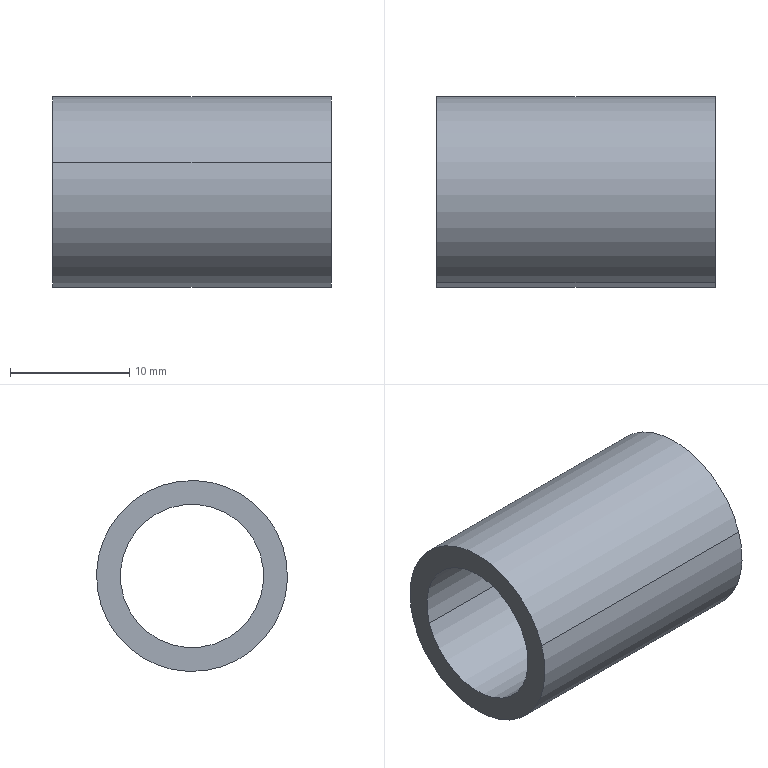Part | STEP file | Completa.sldasm-Part-6_Valor predeterminado | 1 solid | 6 faces | box 23.351 x 16 x 16 mm | volume 2054 mm3 | cylinder 4 | plane 2 | commonest cylinder face diameters 12 x2 16 x2
STEP:
#1=CARTESIAN_POINT('',(0.,0.,0.));
#2=DIRECTION('',(0.,0.,1.));
#3=DIRECTION('',(1.,0.,0.));
#4=AXIS2_PLACEMENT_3D('',#1,#2,#3);
#5=CARTESIAN_POINT('',(-231.995,20.156,-33.743));
#6=VERTEX_POINT('',#5);
#7=CARTESIAN_POINT('',(-255.346,20.156,-33.743));
#8=VERTEX_POINT('',#7);
#9=CARTESIAN_POINT('',(-204.167,20.156,-33.743));
#10=DIRECTION('',(-1.,0.,0.));
#11=VECTOR('',#10,1.);
#12=LINE('',#9,#11);
#13=CARTESIAN_POINT('',(-204.167,25.863,-35.597));
#14=DIRECTION('',(-1.,0.,0.));
#15=DIRECTION('',(0.,-0.9511,0.309));
#16=AXIS2_PLACEMENT_3D('',#13,#14,#15);
#17=CYLINDRICAL_SURFACE('',#16,6.);
#18=CARTESIAN_POINT('',(6.283,0.));
#19=DIRECTION('',(0.,1.));
#20=VECTOR('',#19,1.);
#21=LINE('',#18,#20);
#22=(GEOMETRIC_REPRESENTATION_CONTEXT(2)PARAMETRIC_REPRESENTATION_CONTEXT()REPRESENTATION_CONTEXT('',''));
#23=DEFINITIONAL_REPRESENTATION('',(#21),#22);
#24=PCURVE('',#17,#23);
#25=CARTESIAN_POINT('',(-204.167,25.863,-35.597));
#26=DIRECTION('',(-1.,0.,0.));
#27=DIRECTION('',(0.,-0.9511,0.309));
#28=AXIS2_PLACEMENT_3D('',#25,#26,#27);
#29=CYLINDRICAL_SURFACE('',#28,6.);
#30=CARTESIAN_POINT('',(0.,0.));
#31=DIRECTION('',(0.,1.));
#32=VECTOR('',#31,1.);
#33=LINE('',#30,#32);
#34=(GEOMETRIC_REPRESENTATION_CONTEXT(2)PARAMETRIC_REPRESENTATION_CONTEXT()REPRESENTATION_CONTEXT('',''));
#35=DEFINITIONAL_REPRESENTATION('',(#33),#34);
#36=PCURVE('',#29,#35);
#37=SURFACE_CURVE('',#12,(#24,#36),.PCURVE_S1.);
#38=EDGE_CURVE('',#6,#8,#37,.T.);
#39=ORIENTED_EDGE('',*,*,#38,.T.);
#40=CARTESIAN_POINT('',(-255.346,31.569,-37.451));
#41=VERTEX_POINT('',#40);
#42=CARTESIAN_POINT('',(-255.346,25.863,-35.597));
#43=DIRECTION('',(-1.,0.,0.));
#44=DIRECTION('',(0.,0.9511,-0.309));
#45=AXIS2_PLACEMENT_3D('',#42,#43,#44);
#46=CIRCLE('',#45,6.);
#47=CARTESIAN_POINT('',(3.142,51.179));
#48=DIRECTION('',(1.,0.));
#49=VECTOR('',#48,1.);
#50=LINE('',#47,#49);
#51=(GEOMETRIC_REPRESENTATION_CONTEXT(2)PARAMETRIC_REPRESENTATION_CONTEXT()REPRESENTATION_CONTEXT('',''));
#52=DEFINITIONAL_REPRESENTATION('',(#50),#51);
#53=PCURVE('',#17,#52);
#54=CARTESIAN_POINT('',(-255.346,-11.079,-34.098));
#55=DIRECTION('',(1.,0.,0.));
#56=DIRECTION('',(0.,0.9511,-0.309));
#57=AXIS2_PLACEMENT_3D('',#54,#55,#56);
#58=PLANE('',#57);
#59=CARTESIAN_POINT('',(41.597,9.991));
#60=CARTESIAN_POINT('',(41.597,-0.4016));
#61=CARTESIAN_POINT('',(32.597,4.795));
#62=CARTESIAN_POINT('',(23.597,9.991));
#63=CARTESIAN_POINT('',(32.597,15.187));
#64=CARTESIAN_POINT('',(41.597,20.383));
#65=CARTESIAN_POINT('',(41.597,9.991));
#66=(BOUNDED_CURVE()B_SPLINE_CURVE(2,(#59,#60,#61,#62,#63,#64,#65),.UNSPECIFIED.,.T.,.F.)B_SPLINE_CURVE_WITH_KNOTS((1,2,2,2,2,1),(-2.094,0.,2.094,4.189,6.283,8.378),.UNSPECIFIED.)CURVE()GEOMETRIC_REPRESENTATION_ITEM()RATIONAL_B_SPLINE_CURVE((1.,0.5,1.,0.5,1.,0.5,1.))REPRESENTATION_ITEM(''));
#67=(GEOMETRIC_REPRESENTATION_CONTEXT(2)PARAMETRIC_REPRESENTATION_CONTEXT()REPRESENTATION_CONTEXT('',''));
#68=DEFINITIONAL_REPRESENTATION('',(#66),#67);
#69=PCURVE('',#58,#68);
#70=SURFACE_CURVE('',#46,(#53,#69),.PCURVE_S1.);
#71=EDGE_CURVE('',#41,#8,#70,.T.);
#72=ORIENTED_EDGE('',*,*,#71,.F.);
#73=CARTESIAN_POINT('',(-231.995,31.569,-37.451));
#74=VERTEX_POINT('',#73);
#75=CARTESIAN_POINT('',(-204.167,31.569,-37.451));
#76=DIRECTION('',(-1.,0.,0.));
#77=VECTOR('',#76,1.);
#78=LINE('',#75,#77);
#79=CARTESIAN_POINT('',(3.142,0.));
#80=DIRECTION('',(0.,1.));
#81=VECTOR('',#80,1.);
#82=LINE('',#79,#81);
#83=(GEOMETRIC_REPRESENTATION_CONTEXT(2)PARAMETRIC_REPRESENTATION_CONTEXT()REPRESENTATION_CONTEXT('',''));
#84=DEFINITIONAL_REPRESENTATION('',(#82),#83);
#85=PCURVE('',#17,#84);
#86=CARTESIAN_POINT('',(3.142,0.));
#87=DIRECTION('',(0.,1.));
#88=VECTOR('',#87,1.);
#89=LINE('',#86,#88);
#90=(GEOMETRIC_REPRESENTATION_CONTEXT(2)PARAMETRIC_REPRESENTATION_CONTEXT()REPRESENTATION_CONTEXT('',''));
#91=DEFINITIONAL_REPRESENTATION('',(#89),#90);
#92=PCURVE('',#29,#91);
#93=SURFACE_CURVE('',#78,(#85,#92),.PCURVE_S1.);
#94=EDGE_CURVE('',#74,#41,#93,.T.);
#95=ORIENTED_EDGE('',*,*,#94,.F.);
#96=CARTESIAN_POINT('',(-231.995,25.863,-35.597));
#97=DIRECTION('',(1.,0.,0.));
#98=DIRECTION('',(0.,-0.9511,0.309));
#99=AXIS2_PLACEMENT_3D('',#96,#97,#98);
#100=CIRCLE('',#99,6.);
#101=CARTESIAN_POINT('',(6.283,27.828));
#102=DIRECTION('',(-1.,0.));
#103=VECTOR('',#102,1.);
#104=LINE('',#101,#103);
#105=(GEOMETRIC_REPRESENTATION_CONTEXT(2)PARAMETRIC_REPRESENTATION_CONTEXT()REPRESENTATION_CONTEXT('',''));
#106=DEFINITIONAL_REPRESENTATION('',(#104),#105);
#107=PCURVE('',#17,#106);
#108=CARTESIAN_POINT('',(-231.995,-12.344,-37.989));
#109=DIRECTION('',(-1.,0.,0.));
#110=DIRECTION('',(0.,-0.9511,0.309));
#111=AXIS2_PLACEMENT_3D('',#108,#109,#110);
#112=PLANE('',#111);
#113=CARTESIAN_POINT('',(-29.597,14.082));
#114=CARTESIAN_POINT('',(-29.597,3.69));
#115=CARTESIAN_POINT('',(-38.597,8.886));
#116=CARTESIAN_POINT('',(-47.597,14.082));
#117=CARTESIAN_POINT('',(-38.597,19.278));
#118=CARTESIAN_POINT('',(-29.597,24.474));
#119=CARTESIAN_POINT('',(-29.597,14.082));
#120=(BOUNDED_CURVE()B_SPLINE_CURVE(2,(#113,#114,#115,#116,#117,#118,#119),.UNSPECIFIED.,.T.,.F.)B_SPLINE_CURVE_WITH_KNOTS((1,2,2,2,2,1),(-2.094,0.,2.094,4.189,6.283,8.378),.UNSPECIFIED.)CURVE()GEOMETRIC_REPRESENTATION_ITEM()RATIONAL_B_SPLINE_CURVE((1.,0.5,1.,0.5,1.,0.5,1.))REPRESENTATION_ITEM(''));
#121=(GEOMETRIC_REPRESENTATION_CONTEXT(2)PARAMETRIC_REPRESENTATION_CONTEXT()REPRESENTATION_CONTEXT('',''));
#122=DEFINITIONAL_REPRESENTATION('',(#120),#121);
#123=PCURVE('',#112,#122);
#124=SURFACE_CURVE('',#100,(#107,#123),.PCURVE_S1.);
#125=EDGE_CURVE('',#6,#74,#124,.T.);
#126=ORIENTED_EDGE('',*,*,#125,.F.);
#127=EDGE_LOOP('',(#39,#72,#95,#126));
#128=FACE_BOUND('',#127,.F.);
#129=ADVANCED_FACE('',(#128),#17,.F.);
#130=CARTESIAN_POINT('',(-231.995,33.471,-38.069));
#131=VERTEX_POINT('',#130);
#132=CARTESIAN_POINT('',(-231.995,18.254,-33.125));
#133=VERTEX_POINT('',#132);
#134=CARTESIAN_POINT('',(-231.995,25.863,-35.597));
#135=DIRECTION('',(1.,0.,0.));
#136=DIRECTION('',(0.,-0.9511,0.309));
#137=AXIS2_PLACEMENT_3D('',#134,#135,#136);
#138=CIRCLE('',#137,8.);
#139=CARTESIAN_POINT('',(-204.167,25.863,-35.597));
#140=DIRECTION('',(-1.,0.,0.));
#141=DIRECTION('',(0.,-0.9511,0.309));
#142=AXIS2_PLACEMENT_3D('',#139,#140,#141);
#143=CYLINDRICAL_SURFACE('',#142,8.);
#144=CARTESIAN_POINT('',(6.283,27.828));
#145=DIRECTION('',(-1.,0.));
#146=VECTOR('',#145,1.);
#147=LINE('',#144,#146);
#148=(GEOMETRIC_REPRESENTATION_CONTEXT(2)PARAMETRIC_REPRESENTATION_CONTEXT()REPRESENTATION_CONTEXT('',''));
#149=DEFINITIONAL_REPRESENTATION('',(#147),#148);
#150=PCURVE('',#143,#149);
#151=CARTESIAN_POINT('',(-27.597,14.082));
#152=CARTESIAN_POINT('',(-27.597,0.2255));
#153=CARTESIAN_POINT('',(-39.597,7.154));
#154=CARTESIAN_POINT('',(-51.597,14.082));
#155=CARTESIAN_POINT('',(-39.597,21.01));
#156=CARTESIAN_POINT('',(-27.597,27.938));
#157=CARTESIAN_POINT('',(-27.597,14.082));
#158=(BOUNDED_CURVE()B_SPLINE_CURVE(2,(#151,#152,#153,#154,#155,#156,#157),.UNSPECIFIED.,.T.,.F.)B_SPLINE_CURVE_WITH_KNOTS((1,2,2,2,2,1),(-2.094,0.,2.094,4.189,6.283,8.378),.UNSPECIFIED.)CURVE()GEOMETRIC_REPRESENTATION_ITEM()RATIONAL_B_SPLINE_CURVE((1.,0.5,1.,0.5,1.,0.5,1.))REPRESENTATION_ITEM(''));
#159=(GEOMETRIC_REPRESENTATION_CONTEXT(2)PARAMETRIC_REPRESENTATION_CONTEXT()REPRESENTATION_CONTEXT('',''));
#160=DEFINITIONAL_REPRESENTATION('',(#158),#159);
#161=PCURVE('',#112,#160);
#162=SURFACE_CURVE('',#138,(#150,#161),.PCURVE_S1.);
#163=EDGE_CURVE('',#131,#133,#162,.T.);
#164=ORIENTED_EDGE('',*,*,#163,.F.);
#165=CARTESIAN_POINT('',(-255.346,33.471,-38.069));
#166=VERTEX_POINT('',#165);
#167=CARTESIAN_POINT('',(-204.167,33.471,-38.069));
#168=DIRECTION('',(-1.,0.,0.));
#169=VECTOR('',#168,1.);
#170=LINE('',#167,#169);
#171=CARTESIAN_POINT('',(3.142,0.));
#172=DIRECTION('',(0.,1.));
#173=VECTOR('',#172,1.);
#174=LINE('',#171,#173);
#175=(GEOMETRIC_REPRESENTATION_CONTEXT(2)PARAMETRIC_REPRESENTATION_CONTEXT()REPRESENTATION_CONTEXT('',''));
#176=DEFINITIONAL_REPRESENTATION('',(#174),#175);
#177=PCURVE('',#143,#176);
#178=CARTESIAN_POINT('',(-204.167,25.863,-35.597));
#179=DIRECTION('',(-1.,0.,0.));
#180=DIRECTION('',(0.,-0.9511,0.309));
#181=AXIS2_PLACEMENT_3D('',#178,#179,#180);
#182=CYLINDRICAL_SURFACE('',#181,8.);
#183=CARTESIAN_POINT('',(3.142,0.));
#184=DIRECTION('',(0.,1.));
#185=VECTOR('',#184,1.);
#186=LINE('',#183,#185);
#187=(GEOMETRIC_REPRESENTATION_CONTEXT(2)PARAMETRIC_REPRESENTATION_CONTEXT()REPRESENTATION_CONTEXT('',''));
#188=DEFINITIONAL_REPRESENTATION('',(#186),#187);
#189=PCURVE('',#182,#188);
#190=SURFACE_CURVE('',#170,(#177,#189),.PCURVE_S1.);
#191=EDGE_CURVE('',#131,#166,#190,.T.);
#192=ORIENTED_EDGE('',*,*,#191,.T.);
#193=CARTESIAN_POINT('',(-255.346,18.254,-33.125));
#194=VERTEX_POINT('',#193);
#195=CARTESIAN_POINT('',(-255.346,25.863,-35.597));
#196=DIRECTION('',(-1.,0.,0.));
#197=DIRECTION('',(0.,0.9511,-0.309));
#198=AXIS2_PLACEMENT_3D('',#195,#196,#197);
#199=CIRCLE('',#198,8.);
#200=CARTESIAN_POINT('',(-3.142,51.179));
#201=DIRECTION('',(1.,0.));
#202=VECTOR('',#201,1.);
#203=LINE('',#200,#202);
#204=(GEOMETRIC_REPRESENTATION_CONTEXT(2)PARAMETRIC_REPRESENTATION_CONTEXT()REPRESENTATION_CONTEXT('',''));
#205=DEFINITIONAL_REPRESENTATION('',(#203),#204);
#206=PCURVE('',#143,#205);
#207=CARTESIAN_POINT('',(43.597,9.991));
#208=CARTESIAN_POINT('',(43.597,-3.866));
#209=CARTESIAN_POINT('',(31.597,3.062));
#210=CARTESIAN_POINT('',(19.597,9.991));
#211=CARTESIAN_POINT('',(31.597,16.919));
#212=CARTESIAN_POINT('',(43.597,23.847));
#213=CARTESIAN_POINT('',(43.597,9.991));
#214=(BOUNDED_CURVE()B_SPLINE_CURVE(2,(#207,#208,#209,#210,#211,#212,#213),.UNSPECIFIED.,.T.,.F.)B_SPLINE_CURVE_WITH_KNOTS((1,2,2,2,2,1),(-2.094,0.,2.094,4.189,6.283,8.378),.UNSPECIFIED.)CURVE()GEOMETRIC_REPRESENTATION_ITEM()RATIONAL_B_SPLINE_CURVE((1.,0.5,1.,0.5,1.,0.5,1.))REPRESENTATION_ITEM(''));
#215=(GEOMETRIC_REPRESENTATION_CONTEXT(2)PARAMETRIC_REPRESENTATION_CONTEXT()REPRESENTATION_CONTEXT('',''));
#216=DEFINITIONAL_REPRESENTATION('',(#214),#215);
#217=PCURVE('',#58,#216);
#218=SURFACE_CURVE('',#199,(#206,#217),.PCURVE_S1.);
#219=EDGE_CURVE('',#194,#166,#218,.T.);
#220=ORIENTED_EDGE('',*,*,#219,.F.);
#221=CARTESIAN_POINT('',(-204.167,18.254,-33.125));
#222=DIRECTION('',(-1.,0.,0.));
#223=VECTOR('',#222,1.);
#224=LINE('',#221,#223);
#225=CARTESIAN_POINT('',(0.,0.));
#226=DIRECTION('',(0.,1.));
#227=VECTOR('',#226,1.);
#228=LINE('',#225,#227);
#229=(GEOMETRIC_REPRESENTATION_CONTEXT(2)PARAMETRIC_REPRESENTATION_CONTEXT()REPRESENTATION_CONTEXT('',''));
#230=DEFINITIONAL_REPRESENTATION('',(#228),#229);
#231=PCURVE('',#143,#230);
#232=CARTESIAN_POINT('',(6.283,0.));
#233=DIRECTION('',(0.,1.));
#234=VECTOR('',#233,1.);
#235=LINE('',#232,#234);
#236=(GEOMETRIC_REPRESENTATION_CONTEXT(2)PARAMETRIC_REPRESENTATION_CONTEXT()REPRESENTATION_CONTEXT('',''));
#237=DEFINITIONAL_REPRESENTATION('',(#235),#236);
#238=PCURVE('',#182,#237);
#239=SURFACE_CURVE('',#224,(#231,#238),.PCURVE_S1.);
#240=EDGE_CURVE('',#133,#194,#239,.T.);
#241=ORIENTED_EDGE('',*,*,#240,.F.);
#242=EDGE_LOOP('',(#164,#192,#220,#241));
#243=FACE_BOUND('',#242,.T.);
#244=ADVANCED_FACE('',(#243),#143,.T.);
#245=ORIENTED_EDGE('',*,*,#191,.F.);
#246=CARTESIAN_POINT('',(-231.995,25.863,-35.597));
#247=DIRECTION('',(1.,0.,0.));
#248=DIRECTION('',(0.,-0.9511,0.309));
#249=AXIS2_PLACEMENT_3D('',#246,#247,#248);
#250=CIRCLE('',#249,8.);
#251=CARTESIAN_POINT('',(6.283,27.828));
#252=DIRECTION('',(-1.,0.));
#253=VECTOR('',#252,1.);
#254=LINE('',#251,#253);
#255=(GEOMETRIC_REPRESENTATION_CONTEXT(2)PARAMETRIC_REPRESENTATION_CONTEXT()REPRESENTATION_CONTEXT('',''));
#256=DEFINITIONAL_REPRESENTATION('',(#254),#255);
#257=PCURVE('',#182,#256);
#258=CARTESIAN_POINT('',(-27.597,14.082));
#259=CARTESIAN_POINT('',(-27.597,0.2255));
#260=CARTESIAN_POINT('',(-39.597,7.154));
#261=CARTESIAN_POINT('',(-51.597,14.082));
#262=CARTESIAN_POINT('',(-39.597,21.01));
#263=CARTESIAN_POINT('',(-27.597,27.938));
#264=CARTESIAN_POINT('',(-27.597,14.082));
#265=(BOUNDED_CURVE()B_SPLINE_CURVE(2,(#258,#259,#260,#261,#262,#263,#264),.UNSPECIFIED.,.T.,.F.)B_SPLINE_CURVE_WITH_KNOTS((1,2,2,2,2,1),(-2.094,0.,2.094,4.189,6.283,8.378),.UNSPECIFIED.)CURVE()GEOMETRIC_REPRESENTATION_ITEM()RATIONAL_B_SPLINE_CURVE((1.,0.5,1.,0.5,1.,0.5,1.))REPRESENTATION_ITEM(''));
#266=(GEOMETRIC_REPRESENTATION_CONTEXT(2)PARAMETRIC_REPRESENTATION_CONTEXT()REPRESENTATION_CONTEXT('',''));
#267=DEFINITIONAL_REPRESENTATION('',(#265),#266);
#268=PCURVE('',#112,#267);
#269=SURFACE_CURVE('',#250,(#257,#268),.PCURVE_S1.);
#270=EDGE_CURVE('',#133,#131,#269,.T.);
#271=ORIENTED_EDGE('',*,*,#270,.F.);
#272=ORIENTED_EDGE('',*,*,#240,.T.);
#273=CARTESIAN_POINT('',(-255.346,25.863,-35.597));
#274=DIRECTION('',(-1.,0.,0.));
#275=DIRECTION('',(0.,0.9511,-0.309));
#276=AXIS2_PLACEMENT_3D('',#273,#274,#275);
#277=CIRCLE('',#276,8.);
#278=CARTESIAN_POINT('',(3.142,51.179));
#279=DIRECTION('',(1.,0.));
#280=VECTOR('',#279,1.);
#281=LINE('',#278,#280);
#282=(GEOMETRIC_REPRESENTATION_CONTEXT(2)PARAMETRIC_REPRESENTATION_CONTEXT()REPRESENTATION_CONTEXT('',''));
#283=DEFINITIONAL_REPRESENTATION('',(#281),#282);
#284=PCURVE('',#182,#283);
#285=CARTESIAN_POINT('',(43.597,9.991));
#286=CARTESIAN_POINT('',(43.597,-3.866));
#287=CARTESIAN_POINT('',(31.597,3.062));
#288=CARTESIAN_POINT('',(19.597,9.991));
#289=CARTESIAN_POINT('',(31.597,16.919));
#290=CARTESIAN_POINT('',(43.597,23.847));
#291=CARTESIAN_POINT('',(43.597,9.991));
#292=(BOUNDED_CURVE()B_SPLINE_CURVE(2,(#285,#286,#287,#288,#289,#290,#291),.UNSPECIFIED.,.T.,.F.)B_SPLINE_CURVE_WITH_KNOTS((1,2,2,2,2,1),(-2.094,0.,2.094,4.189,6.283,8.378),.UNSPECIFIED.)CURVE()GEOMETRIC_REPRESENTATION_ITEM()RATIONAL_B_SPLINE_CURVE((1.,0.5,1.,0.5,1.,0.5,1.))REPRESENTATION_ITEM(''));
#293=(GEOMETRIC_REPRESENTATION_CONTEXT(2)PARAMETRIC_REPRESENTATION_CONTEXT()REPRESENTATION_CONTEXT('',''));
#294=DEFINITIONAL_REPRESENTATION('',(#292),#293);
#295=PCURVE('',#58,#294);
#296=SURFACE_CURVE('',#277,(#284,#295),.PCURVE_S1.);
#297=EDGE_CURVE('',#166,#194,#296,.T.);
#298=ORIENTED_EDGE('',*,*,#297,.F.);
#299=EDGE_LOOP('',(#245,#271,#272,#298));
#300=FACE_BOUND('',#299,.T.);
#301=ADVANCED_FACE('',(#300),#182,.T.);
#302=ORIENTED_EDGE('',*,*,#270,.T.);
#303=ORIENTED_EDGE('',*,*,#163,.T.);
#304=EDGE_LOOP('',(#302,#303));
#305=FACE_BOUND('',#304,.T.);
#306=ORIENTED_EDGE('',*,*,#125,.F.);
#307=CARTESIAN_POINT('',(-231.995,25.863,-35.597));
#308=DIRECTION('',(1.,0.,0.));
#309=DIRECTION('',(0.,-0.9511,0.309));
#310=AXIS2_PLACEMENT_3D('',#307,#308,#309);
#311=CIRCLE('',#310,6.);
#312=CARTESIAN_POINT('',(-29.597,14.082));
#313=CARTESIAN_POINT('',(-29.597,3.69));
#314=CARTESIAN_POINT('',(-38.597,8.886));
#315=CARTESIAN_POINT('',(-47.597,14.082));
#316=CARTESIAN_POINT('',(-38.597,19.278));
#317=CARTESIAN_POINT('',(-29.597,24.474));
#318=CARTESIAN_POINT('',(-29.597,14.082));
#319=(BOUNDED_CURVE()B_SPLINE_CURVE(2,(#312,#313,#314,#315,#316,#317,#318),.UNSPECIFIED.,.T.,.F.)B_SPLINE_CURVE_WITH_KNOTS((1,2,2,2,2,1),(-2.094,0.,2.094,4.189,6.283,8.378),.UNSPECIFIED.)CURVE()GEOMETRIC_REPRESENTATION_ITEM()RATIONAL_B_SPLINE_CURVE((1.,0.5,1.,0.5,1.,0.5,1.))REPRESENTATION_ITEM(''));
#320=(GEOMETRIC_REPRESENTATION_CONTEXT(2)PARAMETRIC_REPRESENTATION_CONTEXT()REPRESENTATION_CONTEXT('',''));
#321=DEFINITIONAL_REPRESENTATION('',(#319),#320);
#322=PCURVE('',#112,#321);
#323=CARTESIAN_POINT('',(6.283,27.828));
#324=DIRECTION('',(-1.,0.));
#325=VECTOR('',#324,1.);
#326=LINE('',#323,#325);
#327=(GEOMETRIC_REPRESENTATION_CONTEXT(2)PARAMETRIC_REPRESENTATION_CONTEXT()REPRESENTATION_CONTEXT('',''));
#328=DEFINITIONAL_REPRESENTATION('',(#326),#327);
#329=PCURVE('',#29,#328);
#330=SURFACE_CURVE('',#311,(#322,#329),.PCURVE_S1.);
#331=EDGE_CURVE('',#74,#6,#330,.T.);
#332=ORIENTED_EDGE('',*,*,#331,.F.);
#333=EDGE_LOOP('',(#306,#332));
#334=FACE_BOUND('',#333,.T.);
#335=ADVANCED_FACE('',(#305,#334),#112,.F.);
#336=CARTESIAN_POINT('',(-255.346,25.863,-35.597));
#337=DIRECTION('',(-1.,0.,0.));
#338=DIRECTION('',(0.,0.9511,-0.309));
#339=AXIS2_PLACEMENT_3D('',#336,#337,#338);
#340=CIRCLE('',#339,6.);
#341=CARTESIAN_POINT('',(-3.142,51.179));
#342=DIRECTION('',(1.,0.));
#343=VECTOR('',#342,1.);
#344=LINE('',#341,#343);
#345=(GEOMETRIC_REPRESENTATION_CONTEXT(2)PARAMETRIC_REPRESENTATION_CONTEXT()REPRESENTATION_CONTEXT('',''));
#346=DEFINITIONAL_REPRESENTATION('',(#344),#345);
#347=PCURVE('',#29,#346);
#348=CARTESIAN_POINT('',(41.597,9.991));
#349=CARTESIAN_POINT('',(41.597,-0.4016));
#350=CARTESIAN_POINT('',(32.597,4.795));
#351=CARTESIAN_POINT('',(23.597,9.991));
#352=CARTESIAN_POINT('',(32.597,15.187));
#353=CARTESIAN_POINT('',(41.597,20.383));
#354=CARTESIAN_POINT('',(41.597,9.991));
#355=(BOUNDED_CURVE()B_SPLINE_CURVE(2,(#348,#349,#350,#351,#352,#353,#354),.UNSPECIFIED.,.T.,.F.)B_SPLINE_CURVE_WITH_KNOTS((1,2,2,2,2,1),(-2.094,0.,2.094,4.189,6.283,8.378),.UNSPECIFIED.)CURVE()GEOMETRIC_REPRESENTATION_ITEM()RATIONAL_B_SPLINE_CURVE((1.,0.5,1.,0.5,1.,0.5,1.))REPRESENTATION_ITEM(''));
#356=(GEOMETRIC_REPRESENTATION_CONTEXT(2)PARAMETRIC_REPRESENTATION_CONTEXT()REPRESENTATION_CONTEXT('',''));
#357=DEFINITIONAL_REPRESENTATION('',(#355),#356);
#358=PCURVE('',#58,#357);
#359=SURFACE_CURVE('',#340,(#347,#358),.PCURVE_S1.);
#360=EDGE_CURVE('',#8,#41,#359,.T.);
#361=ORIENTED_EDGE('',*,*,#360,.F.);
#362=ORIENTED_EDGE('',*,*,#38,.F.);
#363=ORIENTED_EDGE('',*,*,#331,.F.);
#364=ORIENTED_EDGE('',*,*,#94,.T.);
#365=EDGE_LOOP('',(#361,#362,#363,#364));
#366=FACE_BOUND('',#365,.F.);
#367=ADVANCED_FACE('',(#366),#29,.F.);
#368=ORIENTED_EDGE('',*,*,#219,.T.);
#369=ORIENTED_EDGE('',*,*,#297,.T.);
#370=EDGE_LOOP('',(#368,#369));
#371=FACE_BOUND('',#370,.T.);
#372=ORIENTED_EDGE('',*,*,#360,.F.);
#373=ORIENTED_EDGE('',*,*,#71,.F.);
#374=EDGE_LOOP('',(#372,#373));
#375=FACE_BOUND('',#374,.T.);
#376=ADVANCED_FACE('',(#371,#375),#58,.F.);
#377=CLOSED_SHELL('',(#129,#244,#301,#335,#367,#376));
#378=MANIFOLD_SOLID_BREP('',#377);
#379=(LENGTH_UNIT()NAMED_UNIT(*)SI_UNIT(.MILLI.,.METRE.));
#380=UNCERTAINTY_MEASURE_WITH_UNIT(LENGTH_MEASURE(0.0000001),#379,'','');
#381=(NAMED_UNIT(*)PLANE_ANGLE_UNIT()SI_UNIT($,.RADIAN.));
#382=(NAMED_UNIT(*)SI_UNIT($,.STERADIAN.)SOLID_ANGLE_UNIT());
#383=(GEOMETRIC_REPRESENTATION_CONTEXT(3)GLOBAL_UNCERTAINTY_ASSIGNED_CONTEXT((#380))GLOBAL_UNIT_ASSIGNED_CONTEXT((#379,#381,#382))REPRESENTATION_CONTEXT('',''));
#384=ADVANCED_BREP_SHAPE_REPRESENTATION('',(#4,#378),#383);